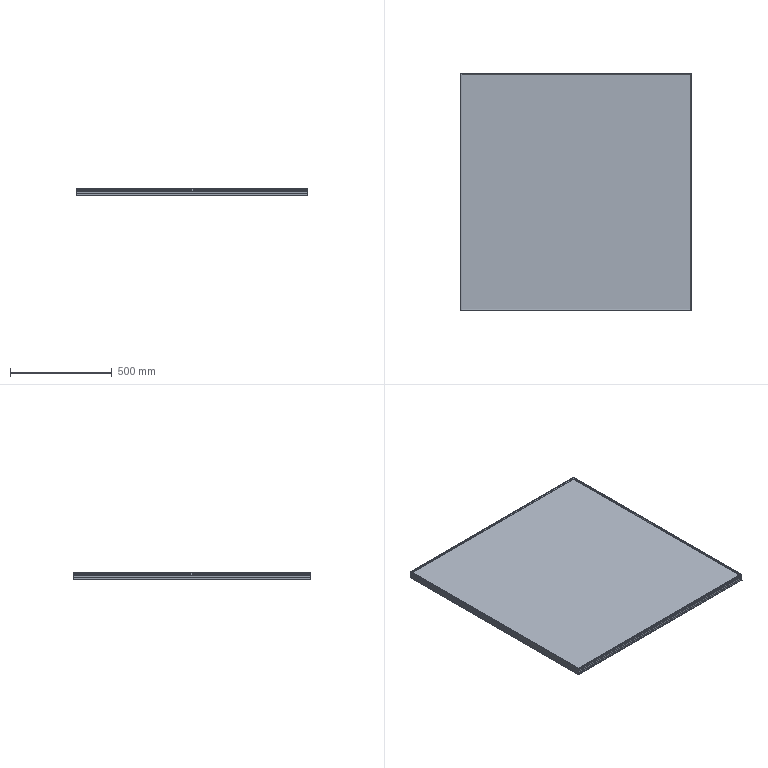Part | 6 solids | 202 faces | box 1140 x 1170 x 36 mm | volume 5732401 mm3 | plane 148 | cylinder 54 | commonest cylinder face diameters 7 x50 5 x4